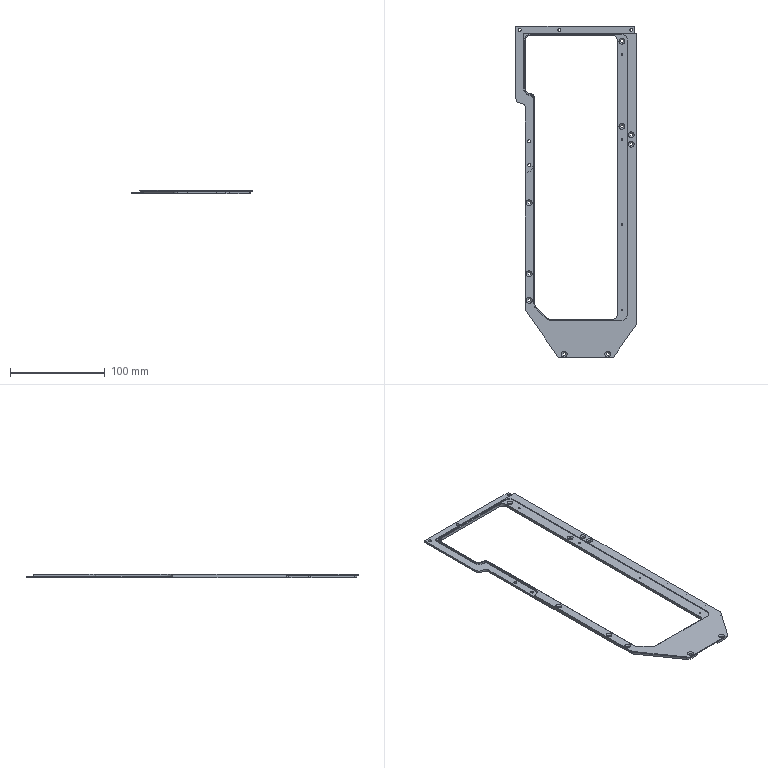CAM job | NX | 3-axis milling, drilling | part box 127 x 351 x 4 mm | stock box 134 x 359 x 4 mm
Tools:
number,name,description,diameter,corner_radius,flute_length,length,flutes
1,CHAMFER_D8-90DEG,倒角D8-90度,8.0,0.0,8.0,60.0,2
2,DRILL_D5.3-62-92,钻刀D5.3-62-92,5.3,0.0,62.0,92.0,2
3,DRILL_D3.2-42-71,钻刀D3.2-42-71,3.2,0.0,42.0,71.0,2
4,D6-18-D6-50-3T-ROUGH,D6-18-D6-50-3T-粗,6.0,0.0,18.0,50.0,2
5,D6-18-D6-50-3T-FINISH,D6-18-D6-50-3T,6.0,0.0,18.0,50.0,3
6,CHAMFER_D3-90DEG,倒角D3-90度,3.0,0.0,5.0,50.0,2
7,DRILL_D1.84-11-D3-40,钻刀D1.84-11-D3-40,1.84,0.0,11.0,12.0,2
8,EXTRUDE_M2-12-D3-39,挤压M2-12-D3-39,2.0,0.0,12.5,14.5,2
0,DRILL_D4.3-54-83,钻刀D4.3-54-83,4.3,0.0,54.0,83.0,2
0,UPPER_ROW_M5-22-D5.5-60,上排M5-22-D5.5-60,5.0,0.0,22.0,25.0,2
0,D2.5,Drilling Tool,2.5,0.0,35.0,50.0,2
Operations:
program,operation,operation_type,tool,method,geometry_group,spindle_rpm,surface_speed,feed_per_tooth,feed_cut,feed_plunge,cut_length_mm,path_length_mm,cut_time_min,machine_time_min
A1,DRILL_HOLES,Operation,CHAMFER_D8-90DEG,METHOD,WORKPIECE,2500.0,62.0,0.05,250.0,0.0,78.4,853.725,0.3136,0.3911
A1,DRILL_HOLES_1_COPY_1,Operation,CHAMFER_D8-90DEG,METHOD,WORKPIECE,2500.0,62.0,0.05,250.0,0.0,9.2,107.498,0.0368,0.0466
A1,DRILL_HOLES_COPY,Operation,DRILL_D5.3-62-92,METHOD,WORKPIECE,3000.0,0.0,0.0,200.0,0.0,133.0,962.925,0.665,0.748
A1,DRILL_HOLES_1_COPY_COPY,Operation,DRILL_D3.2-42-71,METHOD,WORKPIECE,3000.0,0.0,0.0,200.0,0.0,18.0,125.098,0.09,0.1007
A1,PLANAR_MILL_7_COPY_1_COPY,PlanarMilling,CHAMFER_D3-90DEG,METHOD,A-G54,3000.0,28.0,0.1667,300.0,100.0,155.75,277.681,0.5192,0.5314
A1,PLANAR_MILL_7_COPY_1_COPY_COPY,PlanarMilling,CHAMFER_D3-90DEG,METHOD,A-G54,3000.0,28.0,0.1667,300.0,100.0,155.75,277.681,0.5192,0.5314
A2,DRILL_HOLES_1,Operation,CHAMFER_D8-90DEG,METHOD,WORKPIECE,2500.0,62.0,0.05,250.0,0.0,55.2,718.719,0.2208,0.2872
A2,DRILL_HOLES_1_COPY,Operation,DRILL_D3.2-42-71,METHOD,WORKPIECE,3000.0,0.0,0.0,200.0,0.0,108.0,824.319,0.54,0.6116
A2,PLANAR_MILL_8,PlanarMilling,D6-18-D6-50-3T-ROUGH,METHOD,A-G54,3500.0,65.0,0.2143,1500.0,100.0,430.812,737.236,0.2872,0.3179
A2,FLOOR_FACING,VolumeBased25DMillingOperation,D6-18-D6-50-3T-ROUGH,METHOD,A-G54,3500.0,65.0,0.2143,1500.0,100.0,1412.963,1576.689,0.942,0.9583
A2,PLANAR_MILL,PlanarMilling,D6-18-D6-50-3T-ROUGH,METHOD,A-G54,3500.0,65.0,0.2143,1500.0,100.0,155.108,193.908,0.1034,0.1073
A2,PLANAR_MILL_1_COPY_1,PlanarMilling,D6-18-D6-50-3T-ROUGH,METHOD,A-G54,3500.0,65.0,0.2143,1500.0,100.0,4053.411,4782.013,2.702,2.775
A2,PLANAR_MILL_1_COPY_1_COPY,PlanarMilling,D6-18-D6-50-3T-ROUGH,METHOD,A-G54,3500.0,65.0,0.2143,1500.0,100.0,715.0,1458.8,0.4767,0.551
A2,PLANAR_MILL_1,PlanarMilling,D6-18-D6-50-3T-ROUGH,METHOD,A-G54,3500.0,65.0,0.2143,1500.0,100.0,1547.792,2255.895,1.032,1.103
A2,PLANAR_MILL_8_COPY,PlanarMilling,D6-18-D6-50-3T-FINISH,METHOD,A-G54,3500.0,65.0,0.0286,300.0,100.0,66.892,375.092,0.223,0.2538
A2,FLOOR_FACING_COPY,VolumeBased25DMillingOperation,D6-18-D6-50-3T-FINISH,METHOD,A-G54,3500.0,65.0,0.0762,800.0,100.0,461.356,500.356,0.5767,0.5806
A2,PLANAR_MILL_COPY,PlanarMilling,D6-18-D6-50-3T-FINISH,METHOD,A-G54,3500.0,65.0,0.0762,800.0,100.0,155.908,194.908,0.1949,0.1988
A2,PLANAR_MILL_1_COPY_1_COPY_1,PlanarMilling,D6-18-D6-50-3T-FINISH,METHOD,A-G54,3500.0,65.0,0.0762,800.0,100.0,810.768,853.368,1.014,1.018
A2,PLANAR_MILL_1_COPY_1_COPY_COPY,PlanarMilling,D6-18-D6-50-3T-FINISH,METHOD,A-G54,3500.0,65.0,0.0762,800.0,100.0,143.4,186.0,0.1792,0.1835
A2,PLANAR_MILL_1_COPY,PlanarMilling,D6-18-D6-50-3T-FINISH,METHOD,A-G54,3500.0,65.0,0.0762,800.0,100.0,524.181,564.181,0.6552,0.6592
A3,PLANAR_MILL_7,PlanarMilling,CHAMFER_D3-90DEG,METHOD,A-G54,3000.0,28.0,0.1667,1000.0,100.0,859.377,895.377,0.8594,0.863
A3,PLANAR_MILL_7_COPY,PlanarMilling,CHAMFER_D3-90DEG,METHOD,A-G54,3000.0,28.0,0.1667,1000.0,100.0,502.318,546.318,0.5023,0.5067
A3,PLANAR_MILL_9,PlanarMilling,CHAMFER_D3-90DEG,METHOD,A-G54,3000.0,28.0,0.1667,1000.0,100.0,65.235,363.235,0.0652,0.095
B1,DRILLING,Operation,CHAMFER_D8-90DEG,METHOD,B-G55,2500.0,62.0,0.05,250.0,0.0,40.6,590.404,0.1624,0.2174
B1,PLANAR_MILL_2,PlanarMilling,D6-18-D6-50-3T-ROUGH,METHOD,B-G55,3500.0,65.0,0.1429,1000.0,100.0,1178.863,1918.378,1.179,1.253
B1,PLANAR_MILL_2_COPY,PlanarMilling,D6-18-D6-50-3T-ROUGH,METHOD,B-G55,3500.0,65.0,0.1429,1000.0,100.0,120.204,160.004,0.1202,0.1242
B1,PLANAR_MILL_3_COPY,PlanarMilling,D6-18-D6-50-3T-ROUGH,METHOD,B-G55,3500.0,65.0,0.1429,1000.0,100.0,308.0,343.8,0.308,0.3116
B1,PLANAR_MILL_3,PlanarMilling,D6-18-D6-50-3T-ROUGH,METHOD,B-G55,3500.0,65.0,0.1429,1000.0,100.0,793.561,829.361,0.7936,0.7971
B1,PLANAR_MILL_2_COPY_1,PlanarMilling,D6-18-D6-50-3T-FINISH,METHOD,B-G55,3500.0,65.0,0.1429,1000.0,100.0,589.452,864.92,0.5895,0.617
B1,PLANAR_MILL_2_COPY_COPY,PlanarMilling,D6-18-D6-50-3T-FINISH,METHOD,B-G55,3500.0,65.0,0.1429,1000.0,100.0,120.204,160.203,0.1202,0.1242
B1,PLANAR_MILL_3_COPY_1,PlanarMilling,D6-18-D6-50-3T-FINISH,METHOD,B-G55,3500.0,65.0,0.1429,1000.0,100.0,793.989,829.989,0.794,0.7976
B1,PLANAR_MILL_3_COPY_1_COPY,PlanarMilling,D6-18-D6-50-3T-FINISH,METHOD,B-G55,3500.0,65.0,0.1429,1000.0,100.0,789.706,825.706,0.7897,0.7933
B1,PLANAR_MILL_3_COPY_COPY,PlanarMilling,D6-18-D6-50-3T-FINISH,METHOD,B-G55,3500.0,65.0,0.1429,1000.0,100.0,308.0,344.0,0.308,0.3116
B2,DRILLING_2,Operation,CHAMFER_D8-90DEG,METHOD,B-G55,2500.0,62.0,0.04,200.0,0.0,11.6,158.25,0.058,0.0727
B2,DRILLING_1,Operation,CHAMFER_D8-90DEG,METHOD,B-G55,2500.0,62.0,0.04,200.0,0.0,15.2,351.55,0.076,0.1096
B2,DRILLING_3,Operation,DRILL_D1.84-11-D3-40,METHOD,B-G55,1600.0,9.0,0.0312,100.0,0.0,32.0,385.15,0.32,0.3553
B3,PLANAR_MILL_5,PlanarMilling,CHAMFER_D3-90DEG,METHOD,B-G55,3000.0,28.0,0.1667,1000.0,100.0,904.461,942.461,0.9045,0.9083
B3,PLANAR_MILL_5_COPY,PlanarMilling,CHAMFER_D3-90DEG,METHOD,B-G55,3000.0,28.0,0.1667,1000.0,100.0,804.1,841.7,0.8041,0.8079
B3,PLANAR_MILL_6,PlanarMilling,CHAMFER_D3-90DEG,METHOD,B-G55,3000.0,28.0,0.1667,1000.0,100.0,295.462,337.462,0.2955,0.2997
B6,DRILLING_3_COPY,Operation,EXTRUDE_M2-12-D3-39,METHOD,B-G55,300.0,1.0,0.2,120.0,0.0,28.0,377.15,0.2333,0.2682
B6,PLANAR_MILL_4,PlanarMilling,D6-18-D6-50-3T-ROUGH,METHOD,B-G55,3500.0,65.0,0.2143,1500.0,100.0,8012.729,8057.029,5.342,5.346
B6,PLANAR_MILL_4_COPY,PlanarMilling,D6-18-D6-50-3T-FINISH,METHOD,B-G55,3500.0,65.0,0.0762,800.0,100.0,1525.011,1569.611,1.906,1.911
B6,PLANAR_MILL_5_COPY_COPY,PlanarMilling,CHAMFER_D3-90DEG,METHOD,B-G55,3000.0,28.0,0.1667,1000.0,100.0,774.342,814.742,0.7743,0.7784
FIXTURE_1,DRILL_HOLES_COPY_1,Operation,CHAMFER_D8-90DEG,METHOD,WORKPIECE,2500.0,62.0,0.05,250.0,0.0,67.2,808.824,0.2688,0.343
FIXTURE_1,PLANAR_MILL_8_1,PlanarMilling,CHAMFER_D8-90DEG,METHOD,A-G54,3000.0,75.0,0.1667,1000.0,100.0,522.0,556.2,0.522,0.5254
FIXTURE_1,DRILL_HOLES_COPY_COPY,Operation,DRILL_D4.3-54-83,METHOD,WORKPIECE,3000.0,0.0,0.0,200.0,0.0,216.0,1106.424,1.08,1.169
FIXTURE_1,DRILL_HOLES_COPY_COPY_COPY,Operation,UPPER_ROW_M5-22-D5.5-60,METHOD,WORKPIECE,300.0,3.0,0.4,240.0,0.0,156.0,986.424,0.65,0.733
FIXTURE_2,SPOT_FACING,Operation,CHAMFER_D8-90DEG,METHOD,B-G55,2500.0,62.0,0.04,200.0,0.0,17.0,149.779,0.085,0.0983
FIXTURE_2,SPOT_FACING_COPY_1,Operation,CHAMFER_D8-90DEG,METHOD,B-G55,2500.0,62.0,0.04,200.0,0.0,67.5,1001.574,0.3375,0.4309
FIXTURE_2,SPOT_FACING_COPY_1_COPY,Operation,D2.5,METHOD,B-G55,3000.0,23.0,0.0333,200.0,0.0,128.0,1067.24,0.64,0.7339
FIXTURE_2,SPOT_FACING_COPY,Operation,DRILL_D4.3-54-83,METHOD,B-G55,3000.0,23.0,0.0333,200.0,0.0,42.0,199.779,0.21,0.2258
FIXTURE_2,PLANAR_MILL_10,PlanarMilling,D6-18-D6-50-3T-ROUGH,METHOD,B-G55,4500.0,84.0,0.0889,800.0,100.0,716.193,1030.048,0.8952,0.9266
FIXTURE_2,PLANAR_MILL_10_COPY,PlanarMilling,D6-18-D6-50-3T-FINISH,METHOD,B-G55,3500.0,65.0,0.0476,500.0,100.0,43.414,373.414,0.0868,0.1198
FIXTURE_2,PLANAR_MILL_10_COPY_1,PlanarMilling,D6-18-D6-50-3T-ROUGH,METHOD,B-G55,4500.0,84.0,0.0889,800.0,100.0,396.424,442.424,0.4955,0.5001
FIXTURE_2,PLANAR_MILL_10_COPY_COPY,PlanarMilling,D6-18-D6-50-3T-FINISH,METHOD,B-G55,3500.0,65.0,0.0476,500.0,100.0,57.407,113.407,0.1148,0.1204